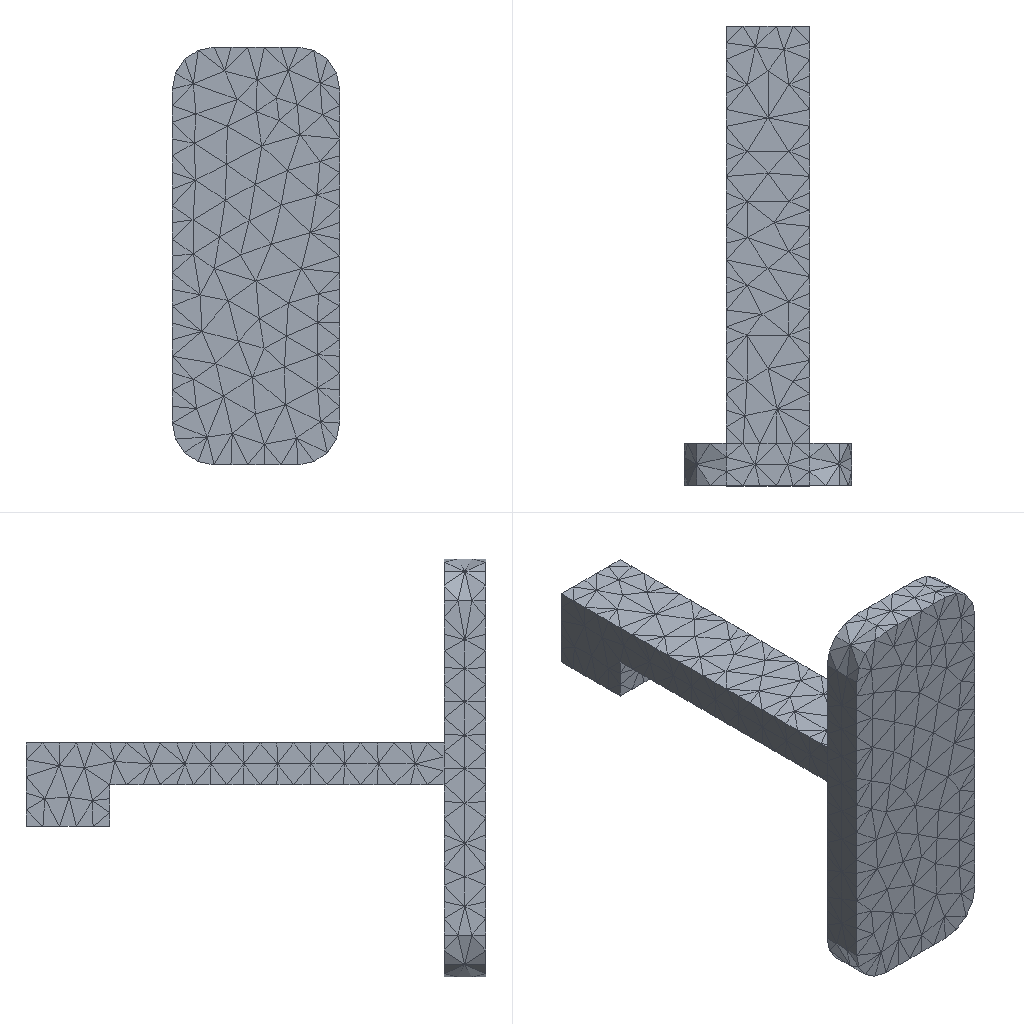Simulation study | ansys workbench
Ansys APDL input file, long lists of numbers shortened:
/batch
/config,noeldb,1     ! force off writing results to database
*get,_wallstrt,active,,time,wall
! ANSYS input file written by Workbench version 2021 R1
! File used for geometry attach:
/title,wbnew--____ (A5)
! ****** Begin Custom Load Command Snippet ******
/COM, ACT Extensions:
/COM,     LSDYNA, 2021.1
/COM,
! ****** End   Custom Load Command Snippet ******
*DIM,_wb_ProjectScratch_dir,string,248
_wb_ProjectScratch_dir(1) = ''
*DIM,_wb_SolverFiles_dir,string,248
_wb_SolverFiles_dir(1) = ''
*DIM,_wb_userfiles_dir,string,248
_wb_userfiles_dir(1) = ''
/com,--- Data in consistent NMM units. See Solving Units in the help system for more information.
/units,MPA
/nopr
/wb,file,start              !  signify a WB generated input file
/prep7
! Turn off shape checking because checks already performed inside WB mesher.
! See help system for more information.
SHPP,OFF,,NOWARN
/nolist
etcon,set             ! allow ANSYS to choose best KEYOP's for 180x elements, resets any applicable keyopt to MAPDL defaults
/com,*********** Nodes for the whole assembly ***********
nblock,3,,3862
(1i9,3e20.9e3)
        1     1.500000000E+01     4.500000000E+01    -3.200000000E+01
! (3510 more lines like these left out)
-1
/wb,elem,start            !  set before creation of elements
/com,*********** Elements for Body 1 "SYS\__" ***********
et,1,187
eblock,19,solid,,1750
(19i9)
        1        1        1        1        0        0        0        0       10        0        1      285      619      395      575     2062     2741     2058     2061
! (3499 more lines like these left out)
-1
/wb,elem,end               !  done creating elements
/com,*********** Send User Defined Coordinate System(s) ***********
csys,0
toffst,273.15,  ! Temperature offset from absolute zero
/com,*********** Set Reference Temperature ***********
tref,22.
/wb,mat,start              !  starting to send materials
/com,*********** Send Materials ***********
Temperature = 'TEMP' ! Temperature
MP,DENS,1,7.85e-09,	! tonne mm^-3
MP,ALPX,1,1.2e-05,	! C^-1
MP,C,1,434000000,	! mm^2 s^-2 C^-1
MP,KXX,1,60.5,	! tonne mm s^-3 C^-1
MP,RSVX,1,0.00017,	! ohm mm
MP,EX,1,200000,	! tonne s^-2 mm^-1
MP,NUXY,1,0.3,
MP,MURX,1,10000,
/wb,mat,end                !  done sending materials
!************************* Model Summary ********************
!SYS\__,	结构钢,	matid,	1
!************************* End Model Summary ********************
! get the diagonal of the bounding box. Needed later for other things
*get,_xmin,node,,mnloc,x
*get,_ymin,node,,mnloc,y
*get,_zmin,node,,mnloc,z
*get,_xmax,node,,mxloc,x
*get,_ymax,node,,mxloc,y
*get,_zmax,node,,mxloc,z
_ASMDIAG=(_xmax-_xmin)*(_xmax-_xmin)+(_ymax-_ymin)*(_ymax-_ymin)+(_zmax-_zmin)*(_zmax-_zmin)
_ASMDIAG=SQRT(_ASMDIAG)
/wb,contact,start          !  starting to send contact
/wb,contact,end            !  done creating contacts
/golist
/wb,load,start             !  starting to send loads
/com,*********** Fixed Supports ***********
CMBLOCK,_FIXEDSU,NODE,      431
(8i10)
       213       216       217       218       219       220       223       226
! (53 more lines like these left out)
cmsel,s,_FIXEDSU
d,all,all
nsel,all
/com,*********** Define Force Using Surface Effect Elements ***********
local,12,0,0.,0.,0.,0.,0.,0.
csys,0
et,2,154
eblock,10,,,28
(15i9)
     2799        2        2        2       12       76      516       77       77     1018     1023       77     1017
! (27 more lines like these left out)
-1
esel,s,type,,2
keyop,2,2,1                ! Apply load in local coordinate system
keyop,2,7,1                ! Use original area so load is constant in large deformation
esel,all
/gst,on,on
fini
*get,_numnode,node,0,count
*get,_numelem,elem,0,count
*get, _MAXELEMNUM, elem, 0, NUM, MAX
*get, _MAXNODENUM, node, 0, NUM, MAX
*get, _MAXELEMTYPE, etyp, 0, NUM, MAX
*get, _MAXREALCONST, real, 0, NUM, MAX
/go
/wb,load,end               !  done creating loads
/com,--- Number of total nodes = %_numnode%
/com,--- Number of contact elements = 28
/com,--- Number of spring elements = 0
/com,--- Number of bearing elements = 0
/com,--- Number of solid elements = 1750
/com,--- Number of condensed parts = 0
/com,--- Number of total elements = %_numelem%
*get,_wallbsol,active,,time,wall
/com,****************************************************************************
/com,*************************    SOLUTION       ********************************
/com,****************************************************************************
/solu
antype,0                   ! static analysis
_thickRatio=  0     ! Ratio of thick parts in the model
eqsl,sparse,,,,,1
cntr,print,1               ! print out contact info and also make no initial contact an error
dmpoption,emat,no             ! Don't combine emat file for DANSYS
dmpoption,esav,no             ! Don't combine esav file for DANSYS
nldiag,cont,iter           ! print out contact info each equilibrium iteration
rescontrol,,none                 ! Do not keep any restart files
/com,****************************************************
/com,******************* SOLVE FOR LS 1 OF 1 ****************
esel,s,type,,2
nsle
sfe,all,1,pres,1,0.
sfe,all,2,pres,1,0.
sfe,all,3,pres,1,5.
nsel,all
esel,all
/nopr
/gopr
/nolist
nsub,1,1,1
time,1.
outres,erase
outres,all,none
outres,nsol,all,
outres,rsol,all
outres,eangl,all
outres,etmp,all
outres,veng,all
outres,strs,all,
outres,epel,all,
outres,eppl,all,
outres,cont,all,
! *********** WB SOLVE COMMAND ***********
! check interactive state
*get,ANSINTER_,active,,int
*if,ANSINTER_,ne,0,then
/eof
*endif
solve
/com *************** Write FE CONNECTORS *********
CEWRITE,file,ce,,INTE
/com,****************************************************
/com,*************** FINISHED SOLVE FOR LS 1 *************
*get,_wallasol,active,,time,wall
/nopr
*get,_numnode,node,0,count
*get,_numelem,elem,0,count
*get, _MAXELEMNUM, elem, 0, NUM, MAX
*get, _MAXNODENUM, node, 0, NUM, MAX,,,INTERNAL
*get, _MAXELEMTYPE, etyp, 0, NUM, MAX
*get, _MAXREALCONST, real, 0, NUM, MAX
/gopr
/post1
xmlo,ENCODING,ISO-8859-1
xmlo,parm
/xml,parm,xml
fini
/gopr
*get,_walldone,active,,time,wall
_preptime=(_wallbsol-_wallstrt)*3600
_solvtime=(_wallasol-_wallbsol)*3600
_posttime=(_walldone-_wallasol)*3600
_totaltim=(_walldone-_wallstrt)*3600
*get,_dlbratio,active,0,solu,dlbr
*get,_combtime,active,0,solu,comb
/com,--- Total number of nodes = %_numnode%
/com,--- Total number of elements = %_numelem%
/com,--- Element load balance ratio = %_dlbratio%
/com,--- Time to combine distributed files = %_combtime%
/wb,file,end               ! done with WB generated input